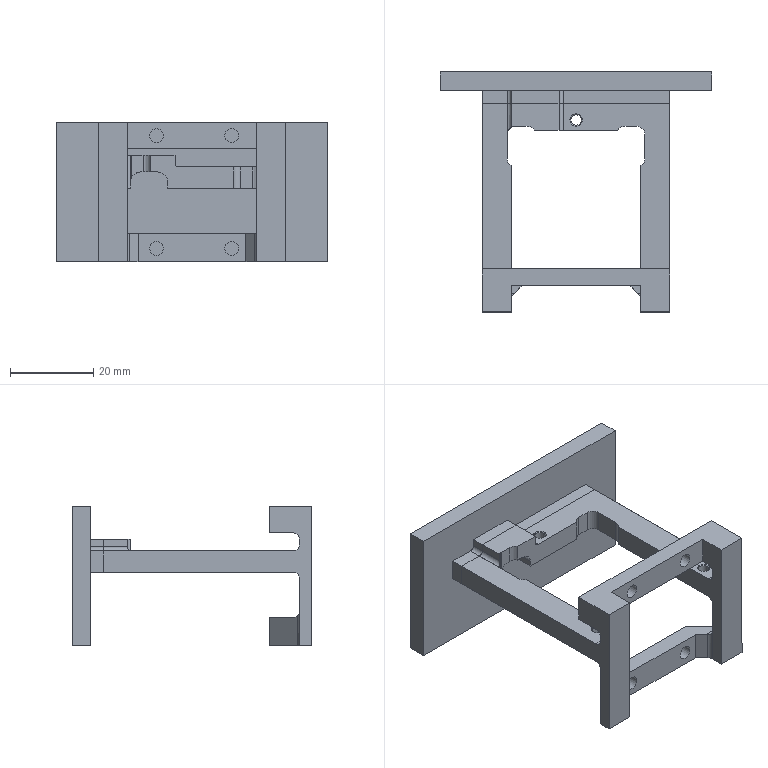Part | 2 solids | 153 faces | box 65 x 57.5 x 33.5 mm | volume 26477 mm3 | plane 81 | cylinder 60 | cone 12 | commonest cylinder face diameters 3 x24 4 x12 3.3 x8 2.5 x6 2 x4 5 x4